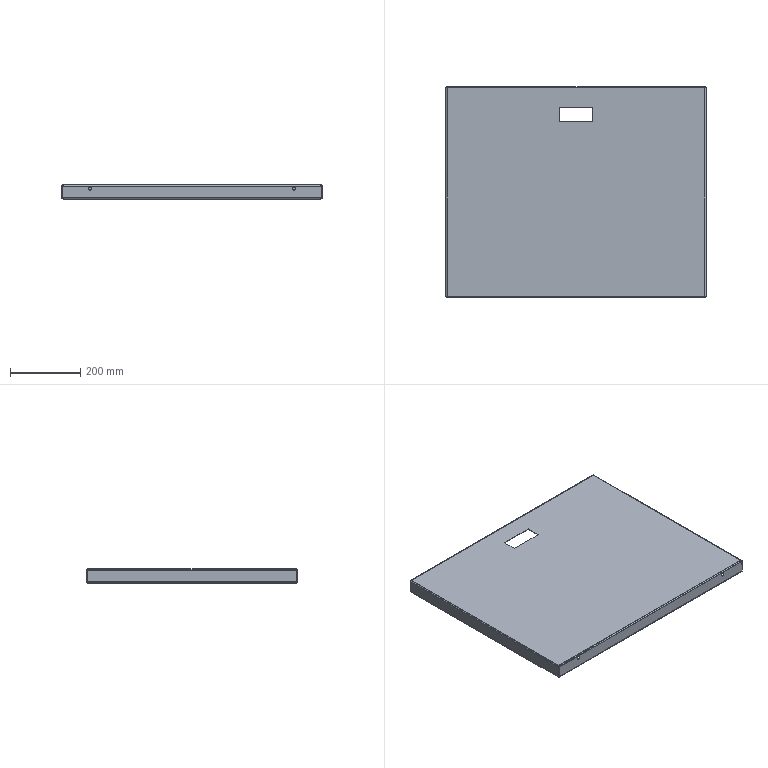Part | SolidWorks | features EdgeFlange 2, FlatPattern 1, HoleWzd 1, SMBaseFlange 1, SheetMetal 1 | 1 solid | 78 faces | box 740 x 600 x 40 mm | volume 876118 mm3 | plane 42 | cylinder 20 | spline 16 | commonest cylinder face diameters 4 x8 7 x8 9 x4